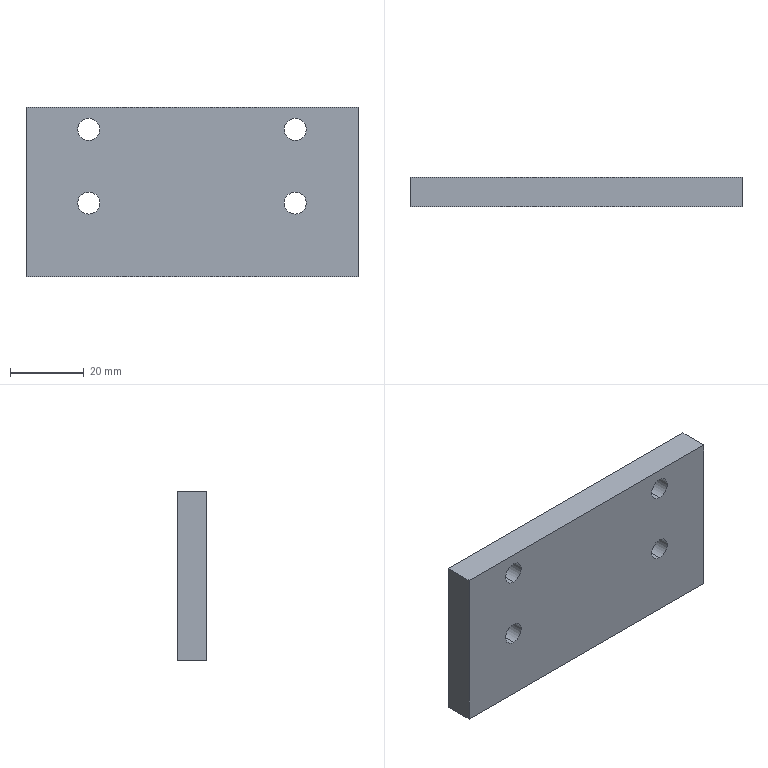Part | STEP file | 0230_205_Plate | 1 solid | 14 faces | box 90 x 8 x 46 mm | volume 32215 mm3 | cylinder 8 | plane 6 | commonest cylinder face diameters 6 x8
STEP:
#1=CARTESIAN_POINT('',(0.,0.,0.));
#2=DIRECTION('',(0.,0.,1.));
#3=DIRECTION('',(1.,0.,0.));
#4=AXIS2_PLACEMENT_3D('',#1,#2,#3);
#5=CARTESIAN_POINT('',(-28.,0.,-23.));
#6=VERTEX_POINT('',#5);
#7=CARTESIAN_POINT('',(-28.,8.,-23.));
#8=VERTEX_POINT('',#7);
#9=CARTESIAN_POINT('',(-28.,8.,-23.));
#10=DIRECTION('',(0.,1.,0.));
#11=VECTOR('',#10,1.);
#12=LINE('',#9,#11);
#13=CARTESIAN_POINT('',(-28.,8.,-26.));
#14=DIRECTION('',(0.,1.,0.));
#15=DIRECTION('',(0.,0.,1.));
#16=AXIS2_PLACEMENT_3D('',#13,#14,#15);
#17=CYLINDRICAL_SURFACE('',#16,3.);
#18=CARTESIAN_POINT('',(6.283,0.));
#19=DIRECTION('',(0.,1.));
#20=VECTOR('',#19,1.);
#21=LINE('',#18,#20);
#22=(GEOMETRIC_REPRESENTATION_CONTEXT(2)PARAMETRIC_REPRESENTATION_CONTEXT()REPRESENTATION_CONTEXT('',''));
#23=DEFINITIONAL_REPRESENTATION('',(#21),#22);
#24=PCURVE('',#17,#23);
#25=CARTESIAN_POINT('',(-28.,8.,-26.));
#26=DIRECTION('',(0.,1.,0.));
#27=DIRECTION('',(0.,0.,1.));
#28=AXIS2_PLACEMENT_3D('',#25,#26,#27);
#29=CYLINDRICAL_SURFACE('',#28,3.);
#30=CARTESIAN_POINT('',(0.,0.));
#31=DIRECTION('',(0.,1.));
#32=VECTOR('',#31,1.);
#33=LINE('',#30,#32);
#34=(GEOMETRIC_REPRESENTATION_CONTEXT(2)PARAMETRIC_REPRESENTATION_CONTEXT()REPRESENTATION_CONTEXT('',''));
#35=DEFINITIONAL_REPRESENTATION('',(#33),#34);
#36=PCURVE('',#29,#35);
#37=SURFACE_CURVE('',#12,(#24,#36),.PCURVE_S1.);
#38=EDGE_CURVE('',#6,#8,#37,.T.);
#39=ORIENTED_EDGE('',*,*,#38,.T.);
#40=CARTESIAN_POINT('',(-28.,8.,-29.));
#41=VERTEX_POINT('',#40);
#42=CARTESIAN_POINT('',(-28.,8.,-26.));
#43=DIRECTION('',(0.,1.,0.));
#44=DIRECTION('',(0.,0.,1.));
#45=AXIS2_PLACEMENT_3D('',#42,#43,#44);
#46=CIRCLE('',#45,3.);
#47=CARTESIAN_POINT('',(0.,0.));
#48=DIRECTION('',(1.,0.));
#49=VECTOR('',#48,1.);
#50=LINE('',#47,#49);
#51=(GEOMETRIC_REPRESENTATION_CONTEXT(2)PARAMETRIC_REPRESENTATION_CONTEXT()REPRESENTATION_CONTEXT('',''));
#52=DEFINITIONAL_REPRESENTATION('',(#50),#51);
#53=PCURVE('',#17,#52);
#54=CARTESIAN_POINT('',(-45.,8.,-46.));
#55=DIRECTION('',(0.,-1.,0.));
#56=DIRECTION('',(0.,0.,-1.));
#57=AXIS2_PLACEMENT_3D('',#54,#55,#56);
#58=PLANE('',#57);
#59=CARTESIAN_POINT('',(-23.,17.));
#60=CARTESIAN_POINT('',(-23.,22.196));
#61=CARTESIAN_POINT('',(-18.5,19.598));
#62=CARTESIAN_POINT('',(-14.,17.));
#63=CARTESIAN_POINT('',(-18.5,14.402));
#64=CARTESIAN_POINT('',(-23.,11.804));
#65=CARTESIAN_POINT('',(-23.,17.));
#66=(BOUNDED_CURVE()B_SPLINE_CURVE(2,(#59,#60,#61,#62,#63,#64,#65),.UNSPECIFIED.,.T.,.F.)B_SPLINE_CURVE_WITH_KNOTS((1,2,2,2,2,1),(-2.094,0.,2.094,4.189,6.283,8.378),.UNSPECIFIED.)CURVE()GEOMETRIC_REPRESENTATION_ITEM()RATIONAL_B_SPLINE_CURVE((1.,0.5,1.,0.5,1.,0.5,1.))REPRESENTATION_ITEM(''));
#67=(GEOMETRIC_REPRESENTATION_CONTEXT(2)PARAMETRIC_REPRESENTATION_CONTEXT()REPRESENTATION_CONTEXT('',''));
#68=DEFINITIONAL_REPRESENTATION('',(#66),#67);
#69=PCURVE('',#58,#68);
#70=SURFACE_CURVE('',#46,(#53,#69),.PCURVE_S1.);
#71=EDGE_CURVE('',#41,#8,#70,.T.);
#72=ORIENTED_EDGE('',*,*,#71,.F.);
#73=CARTESIAN_POINT('',(-28.,0.,-29.));
#74=VERTEX_POINT('',#73);
#75=CARTESIAN_POINT('',(-28.,8.,-29.));
#76=DIRECTION('',(0.,1.,0.));
#77=VECTOR('',#76,1.);
#78=LINE('',#75,#77);
#79=CARTESIAN_POINT('',(3.142,0.));
#80=DIRECTION('',(0.,1.));
#81=VECTOR('',#80,1.);
#82=LINE('',#79,#81);
#83=(GEOMETRIC_REPRESENTATION_CONTEXT(2)PARAMETRIC_REPRESENTATION_CONTEXT()REPRESENTATION_CONTEXT('',''));
#84=DEFINITIONAL_REPRESENTATION('',(#82),#83);
#85=PCURVE('',#17,#84);
#86=CARTESIAN_POINT('',(3.142,0.));
#87=DIRECTION('',(0.,1.));
#88=VECTOR('',#87,1.);
#89=LINE('',#86,#88);
#90=(GEOMETRIC_REPRESENTATION_CONTEXT(2)PARAMETRIC_REPRESENTATION_CONTEXT()REPRESENTATION_CONTEXT('',''));
#91=DEFINITIONAL_REPRESENTATION('',(#89),#90);
#92=PCURVE('',#29,#91);
#93=SURFACE_CURVE('',#78,(#85,#92),.PCURVE_S1.);
#94=EDGE_CURVE('',#74,#41,#93,.T.);
#95=ORIENTED_EDGE('',*,*,#94,.F.);
#96=CARTESIAN_POINT('',(-28.,0.,-26.));
#97=DIRECTION('',(0.,1.,0.));
#98=DIRECTION('',(0.,0.,1.));
#99=AXIS2_PLACEMENT_3D('',#96,#97,#98);
#100=CIRCLE('',#99,3.);
#101=CARTESIAN_POINT('',(0.,-8.));
#102=DIRECTION('',(1.,0.));
#103=VECTOR('',#102,1.);
#104=LINE('',#101,#103);
#105=(GEOMETRIC_REPRESENTATION_CONTEXT(2)PARAMETRIC_REPRESENTATION_CONTEXT()REPRESENTATION_CONTEXT('',''));
#106=DEFINITIONAL_REPRESENTATION('',(#104),#105);
#107=PCURVE('',#17,#106);
#108=CARTESIAN_POINT('',(-45.,0.,-46.));
#109=DIRECTION('',(0.,-1.,0.));
#110=DIRECTION('',(0.,0.,-1.));
#111=AXIS2_PLACEMENT_3D('',#108,#109,#110);
#112=PLANE('',#111);
#113=CARTESIAN_POINT('',(-23.,17.));
#114=CARTESIAN_POINT('',(-23.,22.196));
#115=CARTESIAN_POINT('',(-18.5,19.598));
#116=CARTESIAN_POINT('',(-14.,17.));
#117=CARTESIAN_POINT('',(-18.5,14.402));
#118=CARTESIAN_POINT('',(-23.,11.804));
#119=CARTESIAN_POINT('',(-23.,17.));
#120=(BOUNDED_CURVE()B_SPLINE_CURVE(2,(#113,#114,#115,#116,#117,#118,#119),.UNSPECIFIED.,.T.,.F.)B_SPLINE_CURVE_WITH_KNOTS((1,2,2,2,2,1),(-2.094,0.,2.094,4.189,6.283,8.378),.UNSPECIFIED.)CURVE()GEOMETRIC_REPRESENTATION_ITEM()RATIONAL_B_SPLINE_CURVE((1.,0.5,1.,0.5,1.,0.5,1.))REPRESENTATION_ITEM(''));
#121=(GEOMETRIC_REPRESENTATION_CONTEXT(2)PARAMETRIC_REPRESENTATION_CONTEXT()REPRESENTATION_CONTEXT('',''));
#122=DEFINITIONAL_REPRESENTATION('',(#120),#121);
#123=PCURVE('',#112,#122);
#124=SURFACE_CURVE('',#100,(#107,#123),.PCURVE_S1.);
#125=EDGE_CURVE('',#74,#6,#124,.T.);
#126=ORIENTED_EDGE('',*,*,#125,.T.);
#127=EDGE_LOOP('',(#39,#72,#95,#126));
#128=FACE_BOUND('',#127,.F.);
#129=ADVANCED_FACE('',(#128),#17,.F.);
#130=CARTESIAN_POINT('',(-28.,0.,-3.));
#131=VERTEX_POINT('',#130);
#132=CARTESIAN_POINT('',(-28.,8.,-3.));
#133=VERTEX_POINT('',#132);
#134=CARTESIAN_POINT('',(-28.,8.,-3.));
#135=DIRECTION('',(0.,1.,0.));
#136=VECTOR('',#135,1.);
#137=LINE('',#134,#136);
#138=CARTESIAN_POINT('',(-28.,8.,-6.));
#139=DIRECTION('',(0.,1.,0.));
#140=DIRECTION('',(0.,0.,1.));
#141=AXIS2_PLACEMENT_3D('',#138,#139,#140);
#142=CYLINDRICAL_SURFACE('',#141,3.);
#143=CARTESIAN_POINT('',(6.283,0.));
#144=DIRECTION('',(0.,1.));
#145=VECTOR('',#144,1.);
#146=LINE('',#143,#145);
#147=(GEOMETRIC_REPRESENTATION_CONTEXT(2)PARAMETRIC_REPRESENTATION_CONTEXT()REPRESENTATION_CONTEXT('',''));
#148=DEFINITIONAL_REPRESENTATION('',(#146),#147);
#149=PCURVE('',#142,#148);
#150=CARTESIAN_POINT('',(-28.,8.,-6.));
#151=DIRECTION('',(0.,1.,0.));
#152=DIRECTION('',(0.,0.,1.));
#153=AXIS2_PLACEMENT_3D('',#150,#151,#152);
#154=CYLINDRICAL_SURFACE('',#153,3.);
#155=CARTESIAN_POINT('',(0.,0.));
#156=DIRECTION('',(0.,1.));
#157=VECTOR('',#156,1.);
#158=LINE('',#155,#157);
#159=(GEOMETRIC_REPRESENTATION_CONTEXT(2)PARAMETRIC_REPRESENTATION_CONTEXT()REPRESENTATION_CONTEXT('',''));
#160=DEFINITIONAL_REPRESENTATION('',(#158),#159);
#161=PCURVE('',#154,#160);
#162=SURFACE_CURVE('',#137,(#149,#161),.PCURVE_S1.);
#163=EDGE_CURVE('',#131,#133,#162,.T.);
#164=ORIENTED_EDGE('',*,*,#163,.T.);
#165=CARTESIAN_POINT('',(-28.,8.,-9.));
#166=VERTEX_POINT('',#165);
#167=CARTESIAN_POINT('',(-28.,8.,-6.));
#168=DIRECTION('',(0.,1.,0.));
#169=DIRECTION('',(0.,0.,1.));
#170=AXIS2_PLACEMENT_3D('',#167,#168,#169);
#171=CIRCLE('',#170,3.);
#172=CARTESIAN_POINT('',(0.,0.));
#173=DIRECTION('',(1.,0.));
#174=VECTOR('',#173,1.);
#175=LINE('',#172,#174);
#176=(GEOMETRIC_REPRESENTATION_CONTEXT(2)PARAMETRIC_REPRESENTATION_CONTEXT()REPRESENTATION_CONTEXT('',''));
#177=DEFINITIONAL_REPRESENTATION('',(#175),#176);
#178=PCURVE('',#142,#177);
#179=CARTESIAN_POINT('',(-43.,17.));
#180=CARTESIAN_POINT('',(-43.,22.196));
#181=CARTESIAN_POINT('',(-38.5,19.598));
#182=CARTESIAN_POINT('',(-34.,17.));
#183=CARTESIAN_POINT('',(-38.5,14.402));
#184=CARTESIAN_POINT('',(-43.,11.804));
#185=CARTESIAN_POINT('',(-43.,17.));
#186=(BOUNDED_CURVE()B_SPLINE_CURVE(2,(#179,#180,#181,#182,#183,#184,#185),.UNSPECIFIED.,.T.,.F.)B_SPLINE_CURVE_WITH_KNOTS((1,2,2,2,2,1),(-2.094,0.,2.094,4.189,6.283,8.378),.UNSPECIFIED.)CURVE()GEOMETRIC_REPRESENTATION_ITEM()RATIONAL_B_SPLINE_CURVE((1.,0.5,1.,0.5,1.,0.5,1.))REPRESENTATION_ITEM(''));
#187=(GEOMETRIC_REPRESENTATION_CONTEXT(2)PARAMETRIC_REPRESENTATION_CONTEXT()REPRESENTATION_CONTEXT('',''));
#188=DEFINITIONAL_REPRESENTATION('',(#186),#187);
#189=PCURVE('',#58,#188);
#190=SURFACE_CURVE('',#171,(#178,#189),.PCURVE_S1.);
#191=EDGE_CURVE('',#166,#133,#190,.T.);
#192=ORIENTED_EDGE('',*,*,#191,.F.);
#193=CARTESIAN_POINT('',(-28.,0.,-9.));
#194=VERTEX_POINT('',#193);
#195=CARTESIAN_POINT('',(-28.,8.,-9.));
#196=DIRECTION('',(0.,1.,0.));
#197=VECTOR('',#196,1.);
#198=LINE('',#195,#197);
#199=CARTESIAN_POINT('',(3.142,0.));
#200=DIRECTION('',(0.,1.));
#201=VECTOR('',#200,1.);
#202=LINE('',#199,#201);
#203=(GEOMETRIC_REPRESENTATION_CONTEXT(2)PARAMETRIC_REPRESENTATION_CONTEXT()REPRESENTATION_CONTEXT('',''));
#204=DEFINITIONAL_REPRESENTATION('',(#202),#203);
#205=PCURVE('',#142,#204);
#206=CARTESIAN_POINT('',(3.142,0.));
#207=DIRECTION('',(0.,1.));
#208=VECTOR('',#207,1.);
#209=LINE('',#206,#208);
#210=(GEOMETRIC_REPRESENTATION_CONTEXT(2)PARAMETRIC_REPRESENTATION_CONTEXT()REPRESENTATION_CONTEXT('',''));
#211=DEFINITIONAL_REPRESENTATION('',(#209),#210);
#212=PCURVE('',#154,#211);
#213=SURFACE_CURVE('',#198,(#205,#212),.PCURVE_S1.);
#214=EDGE_CURVE('',#194,#166,#213,.T.);
#215=ORIENTED_EDGE('',*,*,#214,.F.);
#216=CARTESIAN_POINT('',(-28.,0.,-6.));
#217=DIRECTION('',(0.,1.,0.));
#218=DIRECTION('',(0.,0.,1.));
#219=AXIS2_PLACEMENT_3D('',#216,#217,#218);
#220=CIRCLE('',#219,3.);
#221=CARTESIAN_POINT('',(0.,-8.));
#222=DIRECTION('',(1.,0.));
#223=VECTOR('',#222,1.);
#224=LINE('',#221,#223);
#225=(GEOMETRIC_REPRESENTATION_CONTEXT(2)PARAMETRIC_REPRESENTATION_CONTEXT()REPRESENTATION_CONTEXT('',''));
#226=DEFINITIONAL_REPRESENTATION('',(#224),#225);
#227=PCURVE('',#142,#226);
#228=CARTESIAN_POINT('',(-43.,17.));
#229=CARTESIAN_POINT('',(-43.,22.196));
#230=CARTESIAN_POINT('',(-38.5,19.598));
#231=CARTESIAN_POINT('',(-34.,17.));
#232=CARTESIAN_POINT('',(-38.5,14.402));
#233=CARTESIAN_POINT('',(-43.,11.804));
#234=CARTESIAN_POINT('',(-43.,17.));
#235=(BOUNDED_CURVE()B_SPLINE_CURVE(2,(#228,#229,#230,#231,#232,#233,#234),.UNSPECIFIED.,.T.,.F.)B_SPLINE_CURVE_WITH_KNOTS((1,2,2,2,2,1),(-2.094,0.,2.094,4.189,6.283,8.378),.UNSPECIFIED.)CURVE()GEOMETRIC_REPRESENTATION_ITEM()RATIONAL_B_SPLINE_CURVE((1.,0.5,1.,0.5,1.,0.5,1.))REPRESENTATION_ITEM(''));
#236=(GEOMETRIC_REPRESENTATION_CONTEXT(2)PARAMETRIC_REPRESENTATION_CONTEXT()REPRESENTATION_CONTEXT('',''));
#237=DEFINITIONAL_REPRESENTATION('',(#235),#236);
#238=PCURVE('',#112,#237);
#239=SURFACE_CURVE('',#220,(#227,#238),.PCURVE_S1.);
#240=EDGE_CURVE('',#194,#131,#239,.T.);
#241=ORIENTED_EDGE('',*,*,#240,.T.);
#242=EDGE_LOOP('',(#164,#192,#215,#241));
#243=FACE_BOUND('',#242,.F.);
#244=ADVANCED_FACE('',(#243),#142,.F.);
#245=CARTESIAN_POINT('',(28.,0.,-23.));
#246=VERTEX_POINT('',#245);
#247=CARTESIAN_POINT('',(28.,8.,-23.));
#248=VERTEX_POINT('',#247);
#249=CARTESIAN_POINT('',(28.,8.,-23.));
#250=DIRECTION('',(0.,1.,0.));
#251=VECTOR('',#250,1.);
#252=LINE('',#249,#251);
#253=CARTESIAN_POINT('',(28.,8.,-26.));
#254=DIRECTION('',(0.,1.,0.));
#255=DIRECTION('',(0.,0.,1.));
#256=AXIS2_PLACEMENT_3D('',#253,#254,#255);
#257=CYLINDRICAL_SURFACE('',#256,3.);
#258=CARTESIAN_POINT('',(6.283,0.));
#259=DIRECTION('',(0.,1.));
#260=VECTOR('',#259,1.);
#261=LINE('',#258,#260);
#262=(GEOMETRIC_REPRESENTATION_CONTEXT(2)PARAMETRIC_REPRESENTATION_CONTEXT()REPRESENTATION_CONTEXT('',''));
#263=DEFINITIONAL_REPRESENTATION('',(#261),#262);
#264=PCURVE('',#257,#263);
#265=CARTESIAN_POINT('',(28.,8.,-26.));
#266=DIRECTION('',(0.,1.,0.));
#267=DIRECTION('',(0.,0.,1.));
#268=AXIS2_PLACEMENT_3D('',#265,#266,#267);
#269=CYLINDRICAL_SURFACE('',#268,3.);
#270=CARTESIAN_POINT('',(0.,0.));
#271=DIRECTION('',(0.,1.));
#272=VECTOR('',#271,1.);
#273=LINE('',#270,#272);
#274=(GEOMETRIC_REPRESENTATION_CONTEXT(2)PARAMETRIC_REPRESENTATION_CONTEXT()REPRESENTATION_CONTEXT('',''));
#275=DEFINITIONAL_REPRESENTATION('',(#273),#274);
#276=PCURVE('',#269,#275);
#277=SURFACE_CURVE('',#252,(#264,#276),.PCURVE_S1.);
#278=EDGE_CURVE('',#246,#248,#277,.T.);
#279=ORIENTED_EDGE('',*,*,#278,.T.);
#280=CARTESIAN_POINT('',(28.,8.,-29.));
#281=VERTEX_POINT('',#280);
#282=CARTESIAN_POINT('',(28.,8.,-26.));
#283=DIRECTION('',(0.,1.,0.));
#284=DIRECTION('',(0.,0.,1.));
#285=AXIS2_PLACEMENT_3D('',#282,#283,#284);
#286=CIRCLE('',#285,3.);
#287=CARTESIAN_POINT('',(0.,0.));
#288=DIRECTION('',(1.,0.));
#289=VECTOR('',#288,1.);
#290=LINE('',#287,#289);
#291=(GEOMETRIC_REPRESENTATION_CONTEXT(2)PARAMETRIC_REPRESENTATION_CONTEXT()REPRESENTATION_CONTEXT('',''));
#292=DEFINITIONAL_REPRESENTATION('',(#290),#291);
#293=PCURVE('',#257,#292);
#294=CARTESIAN_POINT('',(-23.,73.));
#295=CARTESIAN_POINT('',(-23.,78.196));
#296=CARTESIAN_POINT('',(-18.5,75.598));
#297=CARTESIAN_POINT('',(-14.,73.));
#298=CARTESIAN_POINT('',(-18.5,70.402));
#299=CARTESIAN_POINT('',(-23.,67.804));
#300=CARTESIAN_POINT('',(-23.,73.));
#301=(BOUNDED_CURVE()B_SPLINE_CURVE(2,(#294,#295,#296,#297,#298,#299,#300),.UNSPECIFIED.,.T.,.F.)B_SPLINE_CURVE_WITH_KNOTS((1,2,2,2,2,1),(-2.094,0.,2.094,4.189,6.283,8.378),.UNSPECIFIED.)CURVE()GEOMETRIC_REPRESENTATION_ITEM()RATIONAL_B_SPLINE_CURVE((1.,0.5,1.,0.5,1.,0.5,1.))REPRESENTATION_ITEM(''));
#302=(GEOMETRIC_REPRESENTATION_CONTEXT(2)PARAMETRIC_REPRESENTATION_CONTEXT()REPRESENTATION_CONTEXT('',''));
#303=DEFINITIONAL_REPRESENTATION('',(#301),#302);
#304=PCURVE('',#58,#303);
#305=SURFACE_CURVE('',#286,(#293,#304),.PCURVE_S1.);
#306=EDGE_CURVE('',#281,#248,#305,.T.);
#307=ORIENTED_EDGE('',*,*,#306,.F.);
#308=CARTESIAN_POINT('',(28.,0.,-29.));
#309=VERTEX_POINT('',#308);
#310=CARTESIAN_POINT('',(28.,8.,-29.));
#311=DIRECTION('',(0.,1.,0.));
#312=VECTOR('',#311,1.);
#313=LINE('',#310,#312);
#314=CARTESIAN_POINT('',(3.142,0.));
#315=DIRECTION('',(0.,1.));
#316=VECTOR('',#315,1.);
#317=LINE('',#314,#316);
#318=(GEOMETRIC_REPRESENTATION_CONTEXT(2)PARAMETRIC_REPRESENTATION_CONTEXT()REPRESENTATION_CONTEXT('',''));
#319=DEFINITIONAL_REPRESENTATION('',(#317),#318);
#320=PCURVE('',#257,#319);
#321=CARTESIAN_POINT('',(3.142,0.));
#322=DIRECTION('',(0.,1.));
#323=VECTOR('',#322,1.);
#324=LINE('',#321,#323);
#325=(GEOMETRIC_REPRESENTATION_CONTEXT(2)PARAMETRIC_REPRESENTATION_CONTEXT()REPRESENTATION_CONTEXT('',''));
#326=DEFINITIONAL_REPRESENTATION('',(#324),#325);
#327=PCURVE('',#269,#326);
#328=SURFACE_CURVE('',#313,(#320,#327),.PCURVE_S1.);
#329=EDGE_CURVE('',#309,#281,#328,.T.);
#330=ORIENTED_EDGE('',*,*,#329,.F.);
#331=CARTESIAN_POINT('',(28.,0.,-26.));
#332=DIRECTION('',(0.,1.,0.));
#333=DIRECTION('',(0.,0.,1.));
#334=AXIS2_PLACEMENT_3D('',#331,#332,#333);
#335=CIRCLE('',#334,3.);
#336=CARTESIAN_POINT('',(0.,-8.));
#337=DIRECTION('',(1.,0.));
#338=VECTOR('',#337,1.);
#339=LINE('',#336,#338);
#340=(GEOMETRIC_REPRESENTATION_CONTEXT(2)PARAMETRIC_REPRESENTATION_CONTEXT()REPRESENTATION_CONTEXT('',''));
#341=DEFINITIONAL_REPRESENTATION('',(#339),#340);
#342=PCURVE('',#257,#341);
#343=CARTESIAN_POINT('',(-23.,73.));
#344=CARTESIAN_POINT('',(-23.,78.196));
#345=CARTESIAN_POINT('',(-18.5,75.598));
#346=CARTESIAN_POINT('',(-14.,73.));
#347=CARTESIAN_POINT('',(-18.5,70.402));
#348=CARTESIAN_POINT('',(-23.,67.804));
#349=CARTESIAN_POINT('',(-23.,73.));
#350=(BOUNDED_CURVE()B_SPLINE_CURVE(2,(#343,#344,#345,#346,#347,#348,#349),.UNSPECIFIED.,.T.,.F.)B_SPLINE_CURVE_WITH_KNOTS((1,2,2,2,2,1),(-2.094,0.,2.094,4.189,6.283,8.378),.UNSPECIFIED.)CURVE()GEOMETRIC_REPRESENTATION_ITEM()RATIONAL_B_SPLINE_CURVE((1.,0.5,1.,0.5,1.,0.5,1.))REPRESENTATION_ITEM(''));
#351=(GEOMETRIC_REPRESENTATION_CONTEXT(2)PARAMETRIC_REPRESENTATION_CONTEXT()REPRESENTATION_CONTEXT('',''));
#352=DEFINITIONAL_REPRESENTATION('',(#350),#351);
#353=PCURVE('',#112,#352);
#354=SURFACE_CURVE('',#335,(#342,#353),.PCURVE_S1.);
#355=EDGE_CURVE('',#309,#246,#354,.T.);
#356=ORIENTED_EDGE('',*,*,#355,.T.);
#357=EDGE_LOOP('',(#279,#307,#330,#356));
#358=FACE_BOUND('',#357,.F.);
#359=ADVANCED_FACE('',(#358),#257,.F.);
#360=CARTESIAN_POINT('',(28.,0.,-3.));
#361=VERTEX_POINT('',#360);
#362=CARTESIAN_POINT('',(28.,8.,-3.));
#363=VERTEX_POINT('',#362);
#364=CARTESIAN_POINT('',(28.,8.,-3.));
#365=DIRECTION('',(0.,1.,0.));
#366=VECTOR('',#365,1.);
#367=LINE('',#364,#366);
#368=CARTESIAN_POINT('',(28.,8.,-6.));
#369=DIRECTION('',(0.,1.,0.));
#370=DIRECTION('',(0.,0.,1.));
#371=AXIS2_PLACEMENT_3D('',#368,#369,#370);
#372=CYLINDRICAL_SURFACE('',#371,3.);
#373=CARTESIAN_POINT('',(6.283,0.));
#374=DIRECTION('',(0.,1.));
#375=VECTOR('',#374,1.);
#376=LINE('',#373,#375);
#377=(GEOMETRIC_REPRESENTATION_CONTEXT(2)PARAMETRIC_REPRESENTATION_CONTEXT()REPRESENTATION_CONTEXT('',''));
#378=DEFINITIONAL_REPRESENTATION('',(#376),#377);
#379=PCURVE('',#372,#378);
#380=CARTESIAN_POINT('',(28.,8.,-6.));
#381=DIRECTION('',(0.,1.,0.));
#382=DIRECTION('',(0.,0.,1.));
#383=AXIS2_PLACEMENT_3D('',#380,#381,#382);
#384=CYLINDRICAL_SURFACE('',#383,3.);
#385=CARTESIAN_POINT('',(0.,0.));
#386=DIRECTION('',(0.,1.));
#387=VECTOR('',#386,1.);
#388=LINE('',#385,#387);
#389=(GEOMETRIC_REPRESENTATION_CONTEXT(2)PARAMETRIC_REPRESENTATION_CONTEXT()REPRESENTATION_CONTEXT('',''));
#390=DEFINITIONAL_REPRESENTATION('',(#388),#389);
#391=PCURVE('',#384,#390);
#392=SURFACE_CURVE('',#367,(#379,#391),.PCURVE_S1.);
#393=EDGE_CURVE('',#361,#363,#392,.T.);
#394=ORIENTED_EDGE('',*,*,#393,.T.);
#395=CARTESIAN_POINT('',(28.,8.,-9.));
#396=VERTEX_POINT('',#395);
#397=CARTESIAN_POINT('',(28.,8.,-6.));
#398=DIRECTION('',(0.,1.,0.));
#399=DIRECTION('',(0.,0.,1.));
#400=AXIS2_PLACEMENT_3D('',#397,#398,#399);
#401=CIRCLE('',#400,3.);
#402=CARTESIAN_POINT('',(0.,0.));
#403=DIRECTION('',(1.,0.));
#404=VECTOR('',#403,1.);
#405=LINE('',#402,#404);
#406=(GEOMETRIC_REPRESENTATION_CONTEXT(2)PARAMETRIC_REPRESENTATION_CONTEXT()REPRESENTATION_CONTEXT('',''));
#407=DEFINITIONAL_REPRESENTATION('',(#405),#406);
#408=PCURVE('',#372,#407);
#409=CARTESIAN_POINT('',(-43.,73.));
#410=CARTESIAN_POINT('',(-43.,78.196));
#411=CARTESIAN_POINT('',(-38.5,75.598));
#412=CARTESIAN_POINT('',(-34.,73.));
#413=CARTESIAN_POINT('',(-38.5,70.402));
#414=CARTESIAN_POINT('',(-43.,67.804));
#415=CARTESIAN_POINT('',(-43.,73.));
#416=(BOUNDED_CURVE()B_SPLINE_CURVE(2,(#409,#410,#411,#412,#413,#414,#415),.UNSPECIFIED.,.T.,.F.)B_SPLINE_CURVE_WITH_KNOTS((1,2,2,2,2,1),(-2.094,0.,2.094,4.189,6.283,8.378),.UNSPECIFIED.)CURVE()GEOMETRIC_REPRESENTATION_ITEM()RATIONAL_B_SPLINE_CURVE((1.,0.5,1.,0.5,1.,0.5,1.))REPRESENTATION_ITEM(''));
#417=(GEOMETRIC_REPRESENTATION_CONTEXT(2)PARAMETRIC_REPRESENTATION_CONTEXT()REPRESENTATION_CONTEXT('',''));
#418=DEFINITIONAL_REPRESENTATION('',(#416),#417);
#419=PCURVE('',#58,#418);
#420=SURFACE_CURVE('',#401,(#408,#419),.PCURVE_S1.);
#421=EDGE_CURVE('',#396,#363,#420,.T.);
#422=ORIENTED_EDGE('',*,*,#421,.F.);
#423=CARTESIAN_POINT('',(28.,0.,-9.));
#424=VERTEX_POINT('',#423);
#425=CARTESIAN_POINT('',(28.,8.,-9.));
#426=DIRECTION('',(0.,1.,0.));
#427=VECTOR('',#426,1.);
#428=LINE('',#425,#427);
#429=CARTESIAN_POINT('',(3.142,0.));
#430=DIRECTION('',(0.,1.));
#431=VECTOR('',#430,1.);
#432=LINE('',#429,#431);
#433=(GEOMETRIC_REPRESENTATION_CONTEXT(2)PARAMETRIC_REPRESENTATION_CONTEXT()REPRESENTATION_CONTEXT('',''));
#434=DEFINITIONAL_REPRESENTATION('',(#432),#433);
#435=PCURVE('',#372,#434);
#436=CARTESIAN_POINT('',(3.142,0.));
#437=DIRECTION('',(0.,1.));
#438=VECTOR('',#437,1.);
#439=LINE('',#436,#438);
#440=(GEOMETRIC_REPRESENTATION_CONTEXT(2)PARAMETRIC_REPRESENTATION_CONTEXT()REPRESENTATION_CONTEXT('',''));
#441=DEFINITIONAL_REPRESENTATION('',(#439),#440);
#442=PCURVE('',#384,#441);
#443=SURFACE_CURVE('',#428,(#435,#442),.PCURVE_S1.);
#444=EDGE_CURVE('',#424,#396,#443,.T.);
#445=ORIENTED_EDGE('',*,*,#444,.F.);
#446=CARTESIAN_POINT('',(28.,0.,-6.));
#447=DIRECTION('',(0.,1.,0.));
#448=DIRECTION('',(0.,0.,1.));
#449=AXIS2_PLACEMENT_3D('',#446,#447,#448);
#450=CIRCLE('',#449,3.);
#451=CARTESIAN_POINT('',(0.,-8.));
#452=DIRECTION('',(1.,0.));
#453=VECTOR('',#452,1.);
#454=LINE('',#451,#453);
#455=(GEOMETRIC_REPRESENTATION_CONTEXT(2)PARAMETRIC_REPRESENTATION_CONTEXT()REPRESENTATION_CONTEXT('',''));
#456=DEFINITIONAL_REPRESENTATION('',(#454),#455);
#457=PCURVE('',#372,#456);
#458=CARTESIAN_POINT('',(-43.,73.));
#459=CARTESIAN_POINT('',(-43.,78.196));
#460=CARTESIAN_POINT('',(-38.5,75.598));
#461=CARTESIAN_POINT('',(-34.,73.));
#462=CARTESIAN_POINT('',(-38.5,70.402));
#463=CARTESIAN_POINT('',(-43.,67.804));
#464=CARTESIAN_POINT('',(-43.,73.));
#465=(BOUNDED_CURVE()B_SPLINE_CURVE(2,(#458,#459,#460,#461,#462,#463,#464),.UNSPECIFIED.,.T.,.F.)B_SPLINE_CURVE_WITH_KNOTS((1,2,2,2,2,1),(-2.094,0.,2.094,4.189,6.283,8.378),.UNSPECIFIED.)CURVE()GEOMETRIC_REPRESENTATION_ITEM()RATIONAL_B_SPLINE_CURVE((1.,0.5,1.,0.5,1.,0.5,1.))REPRESENTATION_ITEM(''));
#466=(GEOMETRIC_REPRESENTATION_CONTEXT(2)PARAMETRIC_REPRESENTATION_CONTEXT()REPRESENTATION_CONTEXT('',''));
#467=DEFINITIONAL_REPRESENTATION('',(#465),#466);
#468=PCURVE('',#112,#467);
#469=SURFACE_CURVE('',#450,(#457,#468),.PCURVE_S1.);
#470=EDGE_CURVE('',#424,#361,#469,.T.);
#471=ORIENTED_EDGE('',*,*,#470,.T.);
#472=EDGE_LOOP('',(#394,#422,#445,#471));
#473=FACE_BOUND('',#472,.F.);
#474=ADVANCED_FACE('',(#473),#372,.F.);
#475=CARTESIAN_POINT('',(-45.,0.,-46.));
#476=VERTEX_POINT('',#475);
#477=CARTESIAN_POINT('',(-45.,0.,0.));
#478=VERTEX_POINT('',#477);
#479=CARTESIAN_POINT('',(-45.,0.,0.));
#480=DIRECTION('',(0.,0.,1.));
#481=VECTOR('',#480,1.);
#482=LINE('',#479,#481);
#483=CARTESIAN_POINT('',(-45.,8.,0.));
#484=DIRECTION('',(1.,0.,0.));
#485=DIRECTION('',(0.,0.,-1.));
#486=AXIS2_PLACEMENT_3D('',#483,#484,#485);
#487=PLANE('',#486);
#488=CARTESIAN_POINT('',(0.,-8.));
#489=DIRECTION('',(-1.,0.));
#490=VECTOR('',#489,1.);
#491=LINE('',#488,#490);
#492=(GEOMETRIC_REPRESENTATION_CONTEXT(2)PARAMETRIC_REPRESENTATION_CONTEXT()REPRESENTATION_CONTEXT('',''));
#493=DEFINITIONAL_REPRESENTATION('',(#491),#492);
#494=PCURVE('',#487,#493);
#495=CARTESIAN_POINT('',(-46.,0.));
#496=DIRECTION('',(-1.,0.));
#497=VECTOR('',#496,1.);
#498=LINE('',#495,#497);
#499=(GEOMETRIC_REPRESENTATION_CONTEXT(2)PARAMETRIC_REPRESENTATION_CONTEXT()REPRESENTATION_CONTEXT('',''));
#500=DEFINITIONAL_REPRESENTATION('',(#498),#499);
#501=PCURVE('',#112,#500);
#502=SURFACE_CURVE('',#482,(#494,#501),.PCURVE_S1.);
#503=EDGE_CURVE('',#476,#478,#502,.T.);
#504=ORIENTED_EDGE('',*,*,#503,.T.);
#505=CARTESIAN_POINT('',(-45.,8.,0.));
#506=VERTEX_POINT('',#505);
#507=CARTESIAN_POINT('',(-45.,8.,0.));
#508=DIRECTION('',(0.,-1.,0.));
#509=VECTOR('',#508,1.);
#510=LINE('',#507,#509);
#511=CARTESIAN_POINT('',(0.,0.));
#512=DIRECTION('',(0.,-1.));
#513=VECTOR('',#512,1.);
#514=LINE('',#511,#513);
#515=(GEOMETRIC_REPRESENTATION_CONTEXT(2)PARAMETRIC_REPRESENTATION_CONTEXT()REPRESENTATION_CONTEXT('',''));
#516=DEFINITIONAL_REPRESENTATION('',(#514),#515);
#517=PCURVE('',#487,#516);
#518=CARTESIAN_POINT('',(-45.,8.,0.));
#519=DIRECTION('',(0.,0.,-1.));
#520=DIRECTION('',(-1.,0.,0.));
#521=AXIS2_PLACEMENT_3D('',#518,#519,#520);
#522=PLANE('',#521);
#523=CARTESIAN_POINT('',(0.,0.));
#524=DIRECTION('',(0.,-1.));
#525=VECTOR('',#524,1.);
#526=LINE('',#523,#525);
#527=(GEOMETRIC_REPRESENTATION_CONTEXT(2)PARAMETRIC_REPRESENTATION_CONTEXT()REPRESENTATION_CONTEXT('',''));
#528=DEFINITIONAL_REPRESENTATION('',(#526),#527);
#529=PCURVE('',#522,#528);
#530=SURFACE_CURVE('',#510,(#517,#529),.PCURVE_S1.);
#531=EDGE_CURVE('',#506,#478,#530,.T.);
#532=ORIENTED_EDGE('',*,*,#531,.F.);
#533=CARTESIAN_POINT('',(-45.,8.,-46.));
#534=VERTEX_POINT('',#533);
#535=CARTESIAN_POINT('',(-45.,8.,0.));
#536=DIRECTION('',(0.,0.,1.));
#537=VECTOR('',#536,1.);
#538=LINE('',#535,#537);
#539=CARTESIAN_POINT('',(0.,0.));
#540=DIRECTION('',(-1.,0.));
#541=VECTOR('',#540,1.);
#542=LINE('',#539,#541);
#543=(GEOMETRIC_REPRESENTATION_CONTEXT(2)PARAMETRIC_REPRESENTATION_CONTEXT()REPRESENTATION_CONTEXT('',''));
#544=DEFINITIONAL_REPRESENTATION('',(#542),#543);
#545=PCURVE('',#487,#544);
#546=CARTESIAN_POINT('',(-46.,0.));
#547=DIRECTION('',(-1.,0.));
#548=VECTOR('',#547,1.);
#549=LINE('',#546,#548);
#550=(GEOMETRIC_REPRESENTATION_CONTEXT(2)PARAMETRIC_REPRESENTATION_CONTEXT()REPRESENTATION_CONTEXT('',''));
#551=DEFINITIONAL_REPRESENTATION('',(#549),#550);
#552=PCURVE('',#58,#551);
#553=SURFACE_CURVE('',#538,(#545,#552),.PCURVE_S1.);
#554=EDGE_CURVE('',#534,#506,#553,.T.);
#555=ORIENTED_EDGE('',*,*,#554,.F.);
#556=CARTESIAN_POINT('',(-45.,8.,-46.));
#557=DIRECTION('',(0.,-1.,0.));
#558=VECTOR('',#557,1.);
#559=LINE('',#556,#558);
#560=CARTESIAN_POINT('',(46.,0.));
#561=DIRECTION('',(0.,-1.));
#562=VECTOR('',#561,1.);
#563=LINE('',#560,#562);
#564=(GEOMETRIC_REPRESENTATION_CONTEXT(2)PARAMETRIC_REPRESENTATION_CONTEXT()REPRESENTATION_CONTEXT('',''));
#565=DEFINITIONAL_REPRESENTATION('',(#563),#564);
#566=PCURVE('',#487,#565);
#567=CARTESIAN_POINT('',(-45.,8.,-46.));
#568=DIRECTION('',(0.,0.,1.));
#569=DIRECTION('',(1.,0.,0.));
#570=AXIS2_PLACEMENT_3D('',#567,#568,#569);
#571=PLANE('',#570);
#572=CARTESIAN_POINT('',(0.,0.));
#573=DIRECTION('',(0.,-1.));
#574=VECTOR('',#573,1.);
#575=LINE('',#572,#574);
#576=(GEOMETRIC_REPRESENTATION_CONTEXT(2)PARAMETRIC_REPRESENTATION_CONTEXT()REPRESENTATION_CONTEXT('',''));
#577=DEFINITIONAL_REPRESENTATION('',(#575),#576);
#578=PCURVE('',#571,#577);
#579=SURFACE_CURVE('',#559,(#566,#578),.PCURVE_S1.);
#580=EDGE_CURVE('',#534,#476,#579,.T.);
#581=ORIENTED_EDGE('',*,*,#580,.T.);
#582=EDGE_LOOP('',(#504,#532,#555,#581));
#583=FACE_BOUND('',#582,.T.);
#584=ADVANCED_FACE('',(#583),#487,.F.);
#585=CARTESIAN_POINT('',(45.,0.,0.));
#586=VERTEX_POINT('',#585);
#587=CARTESIAN_POINT('',(-45.,0.,0.));
#588=DIRECTION('',(1.,0.,0.));
#589=VECTOR('',#588,1.);
#590=LINE('',#587,#589);
#591=CARTESIAN_POINT('',(0.,-8.));
#592=DIRECTION('',(-1.,0.));
#593=VECTOR('',#592,1.);
#594=LINE('',#591,#593);
#595=(GEOMETRIC_REPRESENTATION_CONTEXT(2)PARAMETRIC_REPRESENTATION_CONTEXT()REPRESENTATION_CONTEXT('',''));
#596=DEFINITIONAL_REPRESENTATION('',(#594),#595);
#597=PCURVE('',#522,#596);
#598=CARTESIAN_POINT('',(-46.,0.));
#599=DIRECTION('',(0.,1.));
#600=VECTOR('',#599,1.);
#601=LINE('',#598,#600);
#602=(GEOMETRIC_REPRESENTATION_CONTEXT(2)PARAMETRIC_REPRESENTATION_CONTEXT()REPRESENTATION_CONTEXT('',''));
#603=DEFINITIONAL_REPRESENTATION('',(#601),#602);
#604=PCURVE('',#112,#603);
#605=SURFACE_CURVE('',#590,(#597,#604),.PCURVE_S1.);
#606=EDGE_CURVE('',#478,#586,#605,.T.);
#607=ORIENTED_EDGE('',*,*,#606,.T.);
#608=CARTESIAN_POINT('',(45.,8.,0.));
#609=VERTEX_POINT('',#608);
#610=CARTESIAN_POINT('',(45.,8.,0.));
#611=DIRECTION('',(0.,-1.,0.));
#612=VECTOR('',#611,1.);
#613=LINE('',#610,#612);
#614=CARTESIAN_POINT('',(-90.,0.));
#615=DIRECTION('',(0.,-1.));
#616=VECTOR('',#615,1.);
#617=LINE('',#614,#616);
#618=(GEOMETRIC_REPRESENTATION_CONTEXT(2)PARAMETRIC_REPRESENTATION_CONTEXT()REPRESENTATION_CONTEXT('',''));
#619=DEFINITIONAL_REPRESENTATION('',(#617),#618);
#620=PCURVE('',#522,#619);
#621=CARTESIAN_POINT('',(45.,8.,0.));
#622=DIRECTION('',(-1.,0.,0.));
#623=DIRECTION('',(0.,0.,1.));
#624=AXIS2_PLACEMENT_3D('',#621,#622,#623);
#625=PLANE('',#624);
#626=CARTESIAN_POINT('',(0.,0.));
#627=DIRECTION('',(0.,-1.));
#628=VECTOR('',#627,1.);
#629=LINE('',#626,#628);
#630=(GEOMETRIC_REPRESENTATION_CONTEXT(2)PARAMETRIC_REPRESENTATION_CONTEXT()REPRESENTATION_CONTEXT('',''));
#631=DEFINITIONAL_REPRESENTATION('',(#629),#630);
#632=PCURVE('',#625,#631);
#633=SURFACE_CURVE('',#613,(#620,#632),.PCURVE_S1.);
#634=EDGE_CURVE('',#609,#586,#633,.T.);
#635=ORIENTED_EDGE('',*,*,#634,.F.);
#636=CARTESIAN_POINT('',(-45.,8.,0.));
#637=DIRECTION('',(1.,0.,0.));
#638=VECTOR('',#637,1.);
#639=LINE('',#636,#638);
#640=CARTESIAN_POINT('',(0.,0.));
#641=DIRECTION('',(-1.,0.));
#642=VECTOR('',#641,1.);
#643=LINE('',#640,#642);
#644=(GEOMETRIC_REPRESENTATION_CONTEXT(2)PARAMETRIC_REPRESENTATION_CONTEXT()REPRESENTATION_CONTEXT('',''));
#645=DEFINITIONAL_REPRESENTATION('',(#643),#644);
#646=PCURVE('',#522,#645);
#647=CARTESIAN_POINT('',(-46.,0.));
#648=DIRECTION('',(0.,1.));
#649=VECTOR('',#648,1.);
#650=LINE('',#647,#649);
#651=(GEOMETRIC_REPRESENTATION_CONTEXT(2)PARAMETRIC_REPRESENTATION_CONTEXT()REPRESENTATION_CONTEXT('',''));
#652=DEFINITIONAL_REPRESENTATION('',(#650),#651);
#653=PCURVE('',#58,#652);
#654=SURFACE_CURVE('',#639,(#646,#653),.PCURVE_S1.);
#655=EDGE_CURVE('',#506,#609,#654,.T.);
#656=ORIENTED_EDGE('',*,*,#655,.F.);
#657=ORIENTED_EDGE('',*,*,#531,.T.);
#658=EDGE_LOOP('',(#607,#635,#656,#657));
#659=FACE_BOUND('',#658,.T.);
#660=ADVANCED_FACE('',(#659),#522,.F.);
#661=CARTESIAN_POINT('',(45.,0.,-46.));
#662=VERTEX_POINT('',#661);
#663=CARTESIAN_POINT('',(45.,0.,0.));
#664=DIRECTION('',(0.,0.,-1.));
#665=VECTOR('',#664,1.);
#666=LINE('',#663,#665);
#667=CARTESIAN_POINT('',(0.,-8.));
#668=DIRECTION('',(-1.,0.));
#669=VECTOR('',#668,1.);
#670=LINE('',#667,#669);
#671=(GEOMETRIC_REPRESENTATION_CONTEXT(2)PARAMETRIC_REPRESENTATION_CONTEXT()REPRESENTATION_CONTEXT('',''));
#672=DEFINITIONAL_REPRESENTATION('',(#670),#671);
#673=PCURVE('',#625,#672);
#674=CARTESIAN_POINT('',(-46.,90.));
#675=DIRECTION('',(1.,0.));
#676=VECTOR('',#675,1.);
#677=LINE('',#674,#676);
#678=(GEOMETRIC_REPRESENTATION_CONTEXT(2)PARAMETRIC_REPRESENTATION_CONTEXT()REPRESENTATION_CONTEXT('',''));
#679=DEFINITIONAL_REPRESENTATION('',(#677),#678);
#680=PCURVE('',#112,#679);
#681=SURFACE_CURVE('',#666,(#673,#680),.PCURVE_S1.);
#682=EDGE_CURVE('',#586,#662,#681,.T.);
#683=ORIENTED_EDGE('',*,*,#682,.T.);
#684=CARTESIAN_POINT('',(45.,8.,-46.));
#685=VERTEX_POINT('',#684);
#686=CARTESIAN_POINT('',(45.,8.,-46.));
#687=DIRECTION('',(0.,-1.,0.));
#688=VECTOR('',#687,1.);
#689=LINE('',#686,#688);
#690=CARTESIAN_POINT('',(-46.,0.));
#691=DIRECTION('',(0.,-1.));
#692=VECTOR('',#691,1.);
#693=LINE('',#690,#692);
#694=(GEOMETRIC_REPRESENTATION_CONTEXT(2)PARAMETRIC_REPRESENTATION_CONTEXT()REPRESENTATION_CONTEXT('',''));
#695=DEFINITIONAL_REPRESENTATION('',(#693),#694);
#696=PCURVE('',#625,#695);
#697=CARTESIAN_POINT('',(90.,0.));
#698=DIRECTION('',(0.,-1.));
#699=VECTOR('',#698,1.);
#700=LINE('',#697,#699);
#701=(GEOMETRIC_REPRESENTATION_CONTEXT(2)PARAMETRIC_REPRESENTATION_CONTEXT()REPRESENTATION_CONTEXT('',''));
#702=DEFINITIONAL_REPRESENTATION('',(#700),#701);
#703=PCURVE('',#571,#702);
#704=SURFACE_CURVE('',#689,(#696,#703),.PCURVE_S1.);
#705=EDGE_CURVE('',#685,#662,#704,.T.);
#706=ORIENTED_EDGE('',*,*,#705,.F.);
#707=CARTESIAN_POINT('',(45.,8.,0.));
#708=DIRECTION('',(0.,0.,-1.));
#709=VECTOR('',#708,1.);
#710=LINE('',#707,#709);
#711=CARTESIAN_POINT('',(0.,0.));
#712=DIRECTION('',(-1.,0.));
#713=VECTOR('',#712,1.);
#714=LINE('',#711,#713);
#715=(GEOMETRIC_REPRESENTATION_CONTEXT(2)PARAMETRIC_REPRESENTATION_CONTEXT()REPRESENTATION_CONTEXT('',''));
#716=DEFINITIONAL_REPRESENTATION('',(#714),#715);
#717=PCURVE('',#625,#716);
#718=CARTESIAN_POINT('',(-46.,90.));
#719=DIRECTION('',(1.,0.));
#720=VECTOR('',#719,1.);
#721=LINE('',#718,#720);
#722=(GEOMETRIC_REPRESENTATION_CONTEXT(2)PARAMETRIC_REPRESENTATION_CONTEXT()REPRESENTATION_CONTEXT('',''));
#723=DEFINITIONAL_REPRESENTATION('',(#721),#722);
#724=PCURVE('',#58,#723);
#725=SURFACE_CURVE('',#710,(#717,#724),.PCURVE_S1.);
#726=EDGE_CURVE('',#609,#685,#725,.T.);
#727=ORIENTED_EDGE('',*,*,#726,.F.);
#728=ORIENTED_EDGE('',*,*,#634,.T.);
#729=EDGE_LOOP('',(#683,#706,#727,#728));
#730=FACE_BOUND('',#729,.T.);
#731=ADVANCED_FACE('',(#730),#625,.F.);
#732=CARTESIAN_POINT('',(-45.,0.,-46.));
#733=DIRECTION('',(-1.,0.,0.));
#734=VECTOR('',#733,1.);
#735=LINE('',#732,#734);
#736=CARTESIAN_POINT('',(0.,-8.));
#737=DIRECTION('',(-1.,0.));
#738=VECTOR('',#737,1.);
#739=LINE('',#736,#738);
#740=(GEOMETRIC_REPRESENTATION_CONTEXT(2)PARAMETRIC_REPRESENTATION_CONTEXT()REPRESENTATION_CONTEXT('',''));
#741=DEFINITIONAL_REPRESENTATION('',(#739),#740);
#742=PCURVE('',#571,#741);
#743=CARTESIAN_POINT('',(0.,0.));
#744=DIRECTION('',(0.,-1.));
#745=VECTOR('',#744,1.);
#746=LINE('',#743,#745);
#747=(GEOMETRIC_REPRESENTATION_CONTEXT(2)PARAMETRIC_REPRESENTATION_CONTEXT()REPRESENTATION_CONTEXT('',''));
#748=DEFINITIONAL_REPRESENTATION('',(#746),#747);
#749=PCURVE('',#112,#748);
#750=SURFACE_CURVE('',#735,(#742,#749),.PCURVE_S1.);
#751=EDGE_CURVE('',#662,#476,#750,.T.);
#752=ORIENTED_EDGE('',*,*,#751,.T.);
#753=ORIENTED_EDGE('',*,*,#580,.F.);
#754=CARTESIAN_POINT('',(-45.,8.,-46.));
#755=DIRECTION('',(-1.,0.,0.));
#756=VECTOR('',#755,1.);
#757=LINE('',#754,#756);
#758=CARTESIAN_POINT('',(0.,0.));
#759=DIRECTION('',(-1.,0.));
#760=VECTOR('',#759,1.);
#761=LINE('',#758,#760);
#762=(GEOMETRIC_REPRESENTATION_CONTEXT(2)PARAMETRIC_REPRESENTATION_CONTEXT()REPRESENTATION_CONTEXT('',''));
#763=DEFINITIONAL_REPRESENTATION('',(#761),#762);
#764=PCURVE('',#571,#763);
#765=CARTESIAN_POINT('',(0.,0.));
#766=DIRECTION('',(0.,-1.));
#767=VECTOR('',#766,1.);
#768=LINE('',#765,#767);
#769=(GEOMETRIC_REPRESENTATION_CONTEXT(2)PARAMETRIC_REPRESENTATION_CONTEXT()REPRESENTATION_CONTEXT('',''));
#770=DEFINITIONAL_REPRESENTATION('',(#768),#769);
#771=PCURVE('',#58,#770);
#772=SURFACE_CURVE('',#757,(#764,#771),.PCURVE_S1.);
#773=EDGE_CURVE('',#685,#534,#772,.T.);
#774=ORIENTED_EDGE('',*,*,#773,.F.);
#775=ORIENTED_EDGE('',*,*,#705,.T.);
#776=EDGE_LOOP('',(#752,#753,#774,#775));
#777=FACE_BOUND('',#776,.T.);
#778=ADVANCED_FACE('',(#777),#571,.F.);
#779=CARTESIAN_POINT('',(28.,8.,-26.));
#780=DIRECTION('',(0.,1.,0.));
#781=DIRECTION('',(0.,0.,1.));
#782=AXIS2_PLACEMENT_3D('',#779,#780,#781);
#783=CIRCLE('',#782,3.);
#784=CARTESIAN_POINT('',(-23.,73.));
#785=CARTESIAN_POINT('',(-23.,78.196));
#786=CARTESIAN_POINT('',(-18.5,75.598));
#787=CARTESIAN_POINT('',(-14.,73.));
#788=CARTESIAN_POINT('',(-18.5,70.402));
#789=CARTESIAN_POINT('',(-23.,67.804));
#790=CARTESIAN_POINT('',(-23.,73.));
#791=(BOUNDED_CURVE()B_SPLINE_CURVE(2,(#784,#785,#786,#787,#788,#789,#790),.UNSPECIFIED.,.T.,.F.)B_SPLINE_CURVE_WITH_KNOTS((1,2,2,2,2,1),(-2.094,0.,2.094,4.189,6.283,8.378),.UNSPECIFIED.)CURVE()GEOMETRIC_REPRESENTATION_ITEM()RATIONAL_B_SPLINE_CURVE((1.,0.5,1.,0.5,1.,0.5,1.))REPRESENTATION_ITEM(''));
#792=(GEOMETRIC_REPRESENTATION_CONTEXT(2)PARAMETRIC_REPRESENTATION_CONTEXT()REPRESENTATION_CONTEXT('',''));
#793=DEFINITIONAL_REPRESENTATION('',(#791),#792);
#794=PCURVE('',#58,#793);
#795=CARTESIAN_POINT('',(0.,0.));
#796=DIRECTION('',(1.,0.));
#797=VECTOR('',#796,1.);
#798=LINE('',#795,#797);
#799=(GEOMETRIC_REPRESENTATION_CONTEXT(2)PARAMETRIC_REPRESENTATION_CONTEXT()REPRESENTATION_CONTEXT('',''));
#800=DEFINITIONAL_REPRESENTATION('',(#798),#799);
#801=PCURVE('',#269,#800);
#802=SURFACE_CURVE('',#783,(#794,#801),.PCURVE_S1.);
#803=EDGE_CURVE('',#248,#281,#802,.T.);
#804=ORIENTED_EDGE('',*,*,#803,.F.);
#805=ORIENTED_EDGE('',*,*,#306,.F.);
#806=EDGE_LOOP('',(#804,#805));
#807=FACE_BOUND('',#806,.T.);
#808=CARTESIAN_POINT('',(28.,8.,-6.));
#809=DIRECTION('',(0.,1.,0.));
#810=DIRECTION('',(0.,0.,1.));
#811=AXIS2_PLACEMENT_3D('',#808,#809,#810);
#812=CIRCLE('',#811,3.);
#813=CARTESIAN_POINT('',(-43.,73.));
#814=CARTESIAN_POINT('',(-43.,78.196));
#815=CARTESIAN_POINT('',(-38.5,75.598));
#816=CARTESIAN_POINT('',(-34.,73.));
#817=CARTESIAN_POINT('',(-38.5,70.402));
#818=CARTESIAN_POINT('',(-43.,67.804));
#819=CARTESIAN_POINT('',(-43.,73.));
#820=(BOUNDED_CURVE()B_SPLINE_CURVE(2,(#813,#814,#815,#816,#817,#818,#819),.UNSPECIFIED.,.T.,.F.)B_SPLINE_CURVE_WITH_KNOTS((1,2,2,2,2,1),(-2.094,0.,2.094,4.189,6.283,8.378),.UNSPECIFIED.)CURVE()GEOMETRIC_REPRESENTATION_ITEM()RATIONAL_B_SPLINE_CURVE((1.,0.5,1.,0.5,1.,0.5,1.))REPRESENTATION_ITEM(''));
#821=(GEOMETRIC_REPRESENTATION_CONTEXT(2)PARAMETRIC_REPRESENTATION_CONTEXT()REPRESENTATION_CONTEXT('',''));
#822=DEFINITIONAL_REPRESENTATION('',(#820),#821);
#823=PCURVE('',#58,#822);
#824=CARTESIAN_POINT('',(0.,0.));
#825=DIRECTION('',(1.,0.));
#826=VECTOR('',#825,1.);
#827=LINE('',#824,#826);
#828=(GEOMETRIC_REPRESENTATION_CONTEXT(2)PARAMETRIC_REPRESENTATION_CONTEXT()REPRESENTATION_CONTEXT('',''));
#829=DEFINITIONAL_REPRESENTATION('',(#827),#828);
#830=PCURVE('',#384,#829);
#831=SURFACE_CURVE('',#812,(#823,#830),.PCURVE_S1.);
#832=EDGE_CURVE('',#363,#396,#831,.T.);
#833=ORIENTED_EDGE('',*,*,#832,.F.);
#834=ORIENTED_EDGE('',*,*,#421,.F.);
#835=EDGE_LOOP('',(#833,#834));
#836=FACE_BOUND('',#835,.T.);
#837=ORIENTED_EDGE('',*,*,#554,.T.);
#838=ORIENTED_EDGE('',*,*,#655,.T.);
#839=ORIENTED_EDGE('',*,*,#726,.T.);
#840=ORIENTED_EDGE('',*,*,#773,.T.);
#841=EDGE_LOOP('',(#837,#838,#839,#840));
#842=FACE_BOUND('',#841,.T.);
#843=CARTESIAN_POINT('',(-28.,8.,-6.));
#844=DIRECTION('',(0.,1.,0.));
#845=DIRECTION('',(0.,0.,1.));
#846=AXIS2_PLACEMENT_3D('',#843,#844,#845);
#847=CIRCLE('',#846,3.);
#848=CARTESIAN_POINT('',(-43.,17.));
#849=CARTESIAN_POINT('',(-43.,22.196));
#850=CARTESIAN_POINT('',(-38.5,19.598));
#851=CARTESIAN_POINT('',(-34.,17.));
#852=CARTESIAN_POINT('',(-38.5,14.402));
#853=CARTESIAN_POINT('',(-43.,11.804));
#854=CARTESIAN_POINT('',(-43.,17.));
#855=(BOUNDED_CURVE()B_SPLINE_CURVE(2,(#848,#849,#850,#851,#852,#853,#854),.UNSPECIFIED.,.T.,.F.)B_SPLINE_CURVE_WITH_KNOTS((1,2,2,2,2,1),(-2.094,0.,2.094,4.189,6.283,8.378),.UNSPECIFIED.)CURVE()GEOMETRIC_REPRESENTATION_ITEM()RATIONAL_B_SPLINE_CURVE((1.,0.5,1.,0.5,1.,0.5,1.))REPRESENTATION_ITEM(''));
#856=(GEOMETRIC_REPRESENTATION_CONTEXT(2)PARAMETRIC_REPRESENTATION_CONTEXT()REPRESENTATION_CONTEXT('',''));
#857=DEFINITIONAL_REPRESENTATION('',(#855),#856);
#858=PCURVE('',#58,#857);
#859=CARTESIAN_POINT('',(0.,0.));
#860=DIRECTION('',(1.,0.));
#861=VECTOR('',#860,1.);
#862=LINE('',#859,#861);
#863=(GEOMETRIC_REPRESENTATION_CONTEXT(2)PARAMETRIC_REPRESENTATION_CONTEXT()REPRESENTATION_CONTEXT('',''));
#864=DEFINITIONAL_REPRESENTATION('',(#862),#863);
#865=PCURVE('',#154,#864);
#866=SURFACE_CURVE('',#847,(#858,#865),.PCURVE_S1.);
#867=EDGE_CURVE('',#133,#166,#866,.T.);
#868=ORIENTED_EDGE('',*,*,#867,.F.);
#869=ORIENTED_EDGE('',*,*,#191,.F.);
#870=EDGE_LOOP('',(#868,#869));
#871=FACE_BOUND('',#870,.T.);
#872=CARTESIAN_POINT('',(-28.,8.,-26.));
#873=DIRECTION('',(0.,1.,0.));
#874=DIRECTION('',(0.,0.,1.));
#875=AXIS2_PLACEMENT_3D('',#872,#873,#874);
#876=CIRCLE('',#875,3.);
#877=CARTESIAN_POINT('',(-23.,17.));
#878=CARTESIAN_POINT('',(-23.,22.196));
#879=CARTESIAN_POINT('',(-18.5,19.598));
#880=CARTESIAN_POINT('',(-14.,17.));
#881=CARTESIAN_POINT('',(-18.5,14.402));
#882=CARTESIAN_POINT('',(-23.,11.804));
#883=CARTESIAN_POINT('',(-23.,17.));
#884=(BOUNDED_CURVE()B_SPLINE_CURVE(2,(#877,#878,#879,#880,#881,#882,#883),.UNSPECIFIED.,.T.,.F.)B_SPLINE_CURVE_WITH_KNOTS((1,2,2,2,2,1),(-2.094,0.,2.094,4.189,6.283,8.378),.UNSPECIFIED.)CURVE()GEOMETRIC_REPRESENTATION_ITEM()RATIONAL_B_SPLINE_CURVE((1.,0.5,1.,0.5,1.,0.5,1.))REPRESENTATION_ITEM(''));
#885=(GEOMETRIC_REPRESENTATION_CONTEXT(2)PARAMETRIC_REPRESENTATION_CONTEXT()REPRESENTATION_CONTEXT('',''));
#886=DEFINITIONAL_REPRESENTATION('',(#884),#885);
#887=PCURVE('',#58,#886);
#888=CARTESIAN_POINT('',(0.,0.));
#889=DIRECTION('',(1.,0.));
#890=VECTOR('',#889,1.);
#891=LINE('',#888,#890);
#892=(GEOMETRIC_REPRESENTATION_CONTEXT(2)PARAMETRIC_REPRESENTATION_CONTEXT()REPRESENTATION_CONTEXT('',''));
#893=DEFINITIONAL_REPRESENTATION('',(#891),#892);
#894=PCURVE('',#29,#893);
#895=SURFACE_CURVE('',#876,(#887,#894),.PCURVE_S1.);
#896=EDGE_CURVE('',#8,#41,#895,.T.);
#897=ORIENTED_EDGE('',*,*,#896,.F.);
#898=ORIENTED_EDGE('',*,*,#71,.F.);
#899=EDGE_LOOP('',(#897,#898));
#900=FACE_BOUND('',#899,.T.);
#901=ADVANCED_FACE('',(#807,#836,#842,#871,#900),#58,.F.);
#902=CARTESIAN_POINT('',(28.,0.,-26.));
#903=DIRECTION('',(0.,1.,0.));
#904=DIRECTION('',(0.,0.,1.));
#905=AXIS2_PLACEMENT_3D('',#902,#903,#904);
#906=CIRCLE('',#905,3.);
#907=CARTESIAN_POINT('',(-23.,73.));
#908=CARTESIAN_POINT('',(-23.,78.196));
#909=CARTESIAN_POINT('',(-18.5,75.598));
#910=CARTESIAN_POINT('',(-14.,73.));
#911=CARTESIAN_POINT('',(-18.5,70.402));
#912=CARTESIAN_POINT('',(-23.,67.804));
#913=CARTESIAN_POINT('',(-23.,73.));
#914=(BOUNDED_CURVE()B_SPLINE_CURVE(2,(#907,#908,#909,#910,#911,#912,#913),.UNSPECIFIED.,.T.,.F.)B_SPLINE_CURVE_WITH_KNOTS((1,2,2,2,2,1),(-2.094,0.,2.094,4.189,6.283,8.378),.UNSPECIFIED.)CURVE()GEOMETRIC_REPRESENTATION_ITEM()RATIONAL_B_SPLINE_CURVE((1.,0.5,1.,0.5,1.,0.5,1.))REPRESENTATION_ITEM(''));
#915=(GEOMETRIC_REPRESENTATION_CONTEXT(2)PARAMETRIC_REPRESENTATION_CONTEXT()REPRESENTATION_CONTEXT('',''));
#916=DEFINITIONAL_REPRESENTATION('',(#914),#915);
#917=PCURVE('',#112,#916);
#918=CARTESIAN_POINT('',(0.,-8.));
#919=DIRECTION('',(1.,0.));
#920=VECTOR('',#919,1.);
#921=LINE('',#918,#920);
#922=(GEOMETRIC_REPRESENTATION_CONTEXT(2)PARAMETRIC_REPRESENTATION_CONTEXT()REPRESENTATION_CONTEXT('',''));
#923=DEFINITIONAL_REPRESENTATION('',(#921),#922);
#924=PCURVE('',#269,#923);
#925=SURFACE_CURVE('',#906,(#917,#924),.PCURVE_S1.);
#926=EDGE_CURVE('',#246,#309,#925,.T.);
#927=ORIENTED_EDGE('',*,*,#926,.T.);
#928=ORIENTED_EDGE('',*,*,#355,.T.);
#929=EDGE_LOOP('',(#927,#928));
#930=FACE_BOUND('',#929,.T.);
#931=CARTESIAN_POINT('',(28.,0.,-6.));
#932=DIRECTION('',(0.,1.,0.));
#933=DIRECTION('',(0.,0.,1.));
#934=AXIS2_PLACEMENT_3D('',#931,#932,#933);
#935=CIRCLE('',#934,3.);
#936=CARTESIAN_POINT('',(-43.,73.));
#937=CARTESIAN_POINT('',(-43.,78.196));
#938=CARTESIAN_POINT('',(-38.5,75.598));
#939=CARTESIAN_POINT('',(-34.,73.));
#940=CARTESIAN_POINT('',(-38.5,70.402));
#941=CARTESIAN_POINT('',(-43.,67.804));
#942=CARTESIAN_POINT('',(-43.,73.));
#943=(BOUNDED_CURVE()B_SPLINE_CURVE(2,(#936,#937,#938,#939,#940,#941,#942),.UNSPECIFIED.,.T.,.F.)B_SPLINE_CURVE_WITH_KNOTS((1,2,2,2,2,1),(-2.094,0.,2.094,4.189,6.283,8.378),.UNSPECIFIED.)CURVE()GEOMETRIC_REPRESENTATION_ITEM()RATIONAL_B_SPLINE_CURVE((1.,0.5,1.,0.5,1.,0.5,1.))REPRESENTATION_ITEM(''));
#944=(GEOMETRIC_REPRESENTATION_CONTEXT(2)PARAMETRIC_REPRESENTATION_CONTEXT()REPRESENTATION_CONTEXT('',''));
#945=DEFINITIONAL_REPRESENTATION('',(#943),#944);
#946=PCURVE('',#112,#945);
#947=CARTESIAN_POINT('',(0.,-8.));
#948=DIRECTION('',(1.,0.));
#949=VECTOR('',#948,1.);
#950=LINE('',#947,#949);
#951=(GEOMETRIC_REPRESENTATION_CONTEXT(2)PARAMETRIC_REPRESENTATION_CONTEXT()REPRESENTATION_CONTEXT('',''));
#952=DEFINITIONAL_REPRESENTATION('',(#950),#951);
#953=PCURVE('',#384,#952);
#954=SURFACE_CURVE('',#935,(#946,#953),.PCURVE_S1.);
#955=EDGE_CURVE('',#361,#424,#954,.T.);
#956=ORIENTED_EDGE('',*,*,#955,.T.);
#957=ORIENTED_EDGE('',*,*,#470,.T.);
#958=EDGE_LOOP('',(#956,#957));
#959=FACE_BOUND('',#958,.T.);
#960=ORIENTED_EDGE('',*,*,#503,.F.);
#961=ORIENTED_EDGE('',*,*,#751,.F.);
#962=ORIENTED_EDGE('',*,*,#682,.F.);
#963=ORIENTED_EDGE('',*,*,#606,.F.);
#964=EDGE_LOOP('',(#960,#961,#962,#963));
#965=FACE_BOUND('',#964,.T.);
#966=CARTESIAN_POINT('',(-28.,0.,-6.));
#967=DIRECTION('',(0.,1.,0.));
#968=DIRECTION('',(0.,0.,1.));
#969=AXIS2_PLACEMENT_3D('',#966,#967,#968);
#970=CIRCLE('',#969,3.);
#971=CARTESIAN_POINT('',(-43.,17.));
#972=CARTESIAN_POINT('',(-43.,22.196));
#973=CARTESIAN_POINT('',(-38.5,19.598));
#974=CARTESIAN_POINT('',(-34.,17.));
#975=CARTESIAN_POINT('',(-38.5,14.402));
#976=CARTESIAN_POINT('',(-43.,11.804));
#977=CARTESIAN_POINT('',(-43.,17.));
#978=(BOUNDED_CURVE()B_SPLINE_CURVE(2,(#971,#972,#973,#974,#975,#976,#977),.UNSPECIFIED.,.T.,.F.)B_SPLINE_CURVE_WITH_KNOTS((1,2,2,2,2,1),(-2.094,0.,2.094,4.189,6.283,8.378),.UNSPECIFIED.)CURVE()GEOMETRIC_REPRESENTATION_ITEM()RATIONAL_B_SPLINE_CURVE((1.,0.5,1.,0.5,1.,0.5,1.))REPRESENTATION_ITEM(''));
#979=(GEOMETRIC_REPRESENTATION_CONTEXT(2)PARAMETRIC_REPRESENTATION_CONTEXT()REPRESENTATION_CONTEXT('',''));
#980=DEFINITIONAL_REPRESENTATION('',(#978),#979);
#981=PCURVE('',#112,#980);
#982=CARTESIAN_POINT('',(0.,-8.));
#983=DIRECTION('',(1.,0.));
#984=VECTOR('',#983,1.);
#985=LINE('',#982,#984);
#986=(GEOMETRIC_REPRESENTATION_CONTEXT(2)PARAMETRIC_REPRESENTATION_CONTEXT()REPRESENTATION_CONTEXT('',''));
#987=DEFINITIONAL_REPRESENTATION('',(#985),#986);
#988=PCURVE('',#154,#987);
#989=SURFACE_CURVE('',#970,(#981,#988),.PCURVE_S1.);
#990=EDGE_CURVE('',#131,#194,#989,.T.);
#991=ORIENTED_EDGE('',*,*,#990,.T.);
#992=ORIENTED_EDGE('',*,*,#240,.T.);
#993=EDGE_LOOP('',(#991,#992));
#994=FACE_BOUND('',#993,.T.);
#995=CARTESIAN_POINT('',(-28.,0.,-26.));
#996=DIRECTION('',(0.,1.,0.));
#997=DIRECTION('',(0.,0.,1.));
#998=AXIS2_PLACEMENT_3D('',#995,#996,#997);
#999=CIRCLE('',#998,3.);
#1000=CARTESIAN_POINT('',(-23.,17.));
#1001=CARTESIAN_POINT('',(-23.,22.196));
#1002=CARTESIAN_POINT('',(-18.5,19.598));
#1003=CARTESIAN_POINT('',(-14.,17.));
#1004=CARTESIAN_POINT('',(-18.5,14.402));
#1005=CARTESIAN_POINT('',(-23.,11.804));
#1006=CARTESIAN_POINT('',(-23.,17.));
#1007=(BOUNDED_CURVE()B_SPLINE_CURVE(2,(#1000,#1001,#1002,#1003,#1004,#1005,#1006),.UNSPECIFIED.,.T.,.F.)B_SPLINE_CURVE_WITH_KNOTS((1,2,2,2,2,1),(-2.094,0.,2.094,4.189,6.283,8.378),.UNSPECIFIED.)CURVE()GEOMETRIC_REPRESENTATION_ITEM()RATIONAL_B_SPLINE_CURVE((1.,0.5,1.,0.5,1.,0.5,1.))REPRESENTATION_ITEM(''));
#1008=(GEOMETRIC_REPRESENTATION_CONTEXT(2)PARAMETRIC_REPRESENTATION_CONTEXT()REPRESENTATION_CONTEXT('',''));
#1009=DEFINITIONAL_REPRESENTATION('',(#1007),#1008);
#1010=PCURVE('',#112,#1009);
#1011=CARTESIAN_POINT('',(0.,-8.));
#1012=DIRECTION('',(1.,0.));
#1013=VECTOR('',#1012,1.);
#1014=LINE('',#1011,#1013);
#1015=(GEOMETRIC_REPRESENTATION_CONTEXT(2)PARAMETRIC_REPRESENTATION_CONTEXT()REPRESENTATION_CONTEXT('',''));
#1016=DEFINITIONAL_REPRESENTATION('',(#1014),#1015);
#1017=PCURVE('',#29,#1016);
#1018=SURFACE_CURVE('',#999,(#1010,#1017),.PCURVE_S1.);
#1019=EDGE_CURVE('',#6,#74,#1018,.T.);
#1020=ORIENTED_EDGE('',*,*,#1019,.T.);
#1021=ORIENTED_EDGE('',*,*,#125,.T.);
#1022=EDGE_LOOP('',(#1020,#1021));
#1023=FACE_BOUND('',#1022,.T.);
#1024=ADVANCED_FACE('',(#930,#959,#965,#994,#1023),#112,.T.);
#1025=ORIENTED_EDGE('',*,*,#832,.F.);
#1026=ORIENTED_EDGE('',*,*,#393,.F.);
#1027=ORIENTED_EDGE('',*,*,#955,.T.);
#1028=ORIENTED_EDGE('',*,*,#444,.T.);
#1029=EDGE_LOOP('',(#1025,#1026,#1027,#1028));
#1030=FACE_BOUND('',#1029,.F.);
#1031=ADVANCED_FACE('',(#1030),#384,.F.);
#1032=ORIENTED_EDGE('',*,*,#803,.F.);
#1033=ORIENTED_EDGE('',*,*,#278,.F.);
#1034=ORIENTED_EDGE('',*,*,#926,.T.);
#1035=ORIENTED_EDGE('',*,*,#329,.T.);
#1036=EDGE_LOOP('',(#1032,#1033,#1034,#1035));
#1037=FACE_BOUND('',#1036,.F.);
#1038=ADVANCED_FACE('',(#1037),#269,.F.);
#1039=ORIENTED_EDGE('',*,*,#867,.F.);
#1040=ORIENTED_EDGE('',*,*,#163,.F.);
#1041=ORIENTED_EDGE('',*,*,#990,.T.);
#1042=ORIENTED_EDGE('',*,*,#214,.T.);
#1043=EDGE_LOOP('',(#1039,#1040,#1041,#1042));
#1044=FACE_BOUND('',#1043,.F.);
#1045=ADVANCED_FACE('',(#1044),#154,.F.);
#1046=ORIENTED_EDGE('',*,*,#896,.F.);
#1047=ORIENTED_EDGE('',*,*,#38,.F.);
#1048=ORIENTED_EDGE('',*,*,#1019,.T.);
#1049=ORIENTED_EDGE('',*,*,#94,.T.);
#1050=EDGE_LOOP('',(#1046,#1047,#1048,#1049));
#1051=FACE_BOUND('',#1050,.F.);
#1052=ADVANCED_FACE('',(#1051),#29,.F.);
#1053=CLOSED_SHELL('',(#129,#244,#359,#474,#584,#660,#731,#778,#901,#1024,#1031,#1038,#1045,#1052));
#1054=MANIFOLD_SOLID_BREP('',#1053);
#1055=(LENGTH_UNIT()NAMED_UNIT(*)SI_UNIT(.MILLI.,.METRE.));
#1056=UNCERTAINTY_MEASURE_WITH_UNIT(LENGTH_MEASURE(0.0000001),#1055,'','');
#1057=(NAMED_UNIT(*)PLANE_ANGLE_UNIT()SI_UNIT($,.RADIAN.));
#1058=(NAMED_UNIT(*)SI_UNIT($,.STERADIAN.)SOLID_ANGLE_UNIT());
#1059=(GEOMETRIC_REPRESENTATION_CONTEXT(3)GLOBAL_UNCERTAINTY_ASSIGNED_CONTEXT((#1056))GLOBAL_UNIT_ASSIGNED_CONTEXT((#1055,#1057,#1058))REPRESENTATION_CONTEXT('',''));
#1060=ADVANCED_BREP_SHAPE_REPRESENTATION('',(#4,#1054),#1059);